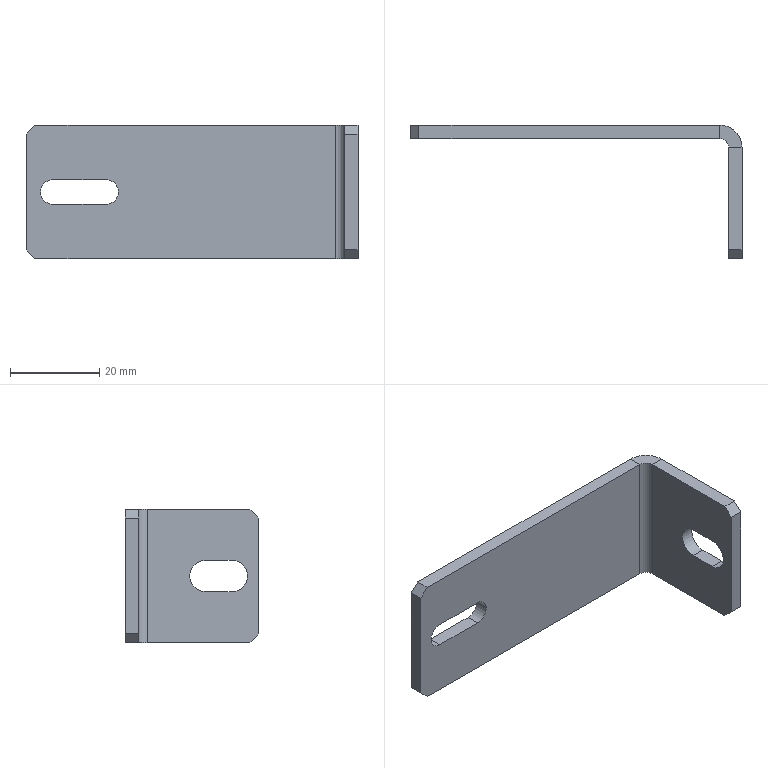Part | NX | features BREP 1 | 1 solid | 26 faces | box 74.5 x 30 x 30 mm | volume 8465 mm3 | plane 20 | cylinder 6 | commonest cylinder face diameters 5.5 x2 7 x2 4 x1 10 x1
STEP:
#1=CARTESIAN_POINT('',(74.5,-30.,-13.));
#2=VERTEX_POINT('',#1);
#3=CARTESIAN_POINT('',(74.5,-28.,-15.));
#4=VERTEX_POINT('',#3);
#5=CARTESIAN_POINT('',(74.5,-29.,-14.));
#6=DIRECTION('',(0.,0.7071,-0.7071));
#7=VECTOR('',#6,1000.);
#8=LINE('',#5,#7);
#9=EDGE_CURVE('',#2,#4,#8,.T.);
#10=ORIENTED_EDGE('',*,*,#9,.F.);
#11=CARTESIAN_POINT('',(71.5,-30.,-13.));
#12=VERTEX_POINT('',#11);
#13=CARTESIAN_POINT('',(74.5,-30.,-13.));
#14=DIRECTION('',(1.,0.,0.));
#15=VECTOR('',#14,1000.);
#16=LINE('',#13,#15);
#17=EDGE_CURVE('',#12,#2,#16,.T.);
#18=ORIENTED_EDGE('',*,*,#17,.F.);
#19=CARTESIAN_POINT('',(71.5,-28.,-15.));
#20=VERTEX_POINT('',#19);
#21=CARTESIAN_POINT('',(71.5,-28.,-15.));
#22=DIRECTION('',(0.,-0.7071,0.7071));
#23=VECTOR('',#22,1000.);
#24=LINE('',#21,#23);
#25=EDGE_CURVE('',#20,#12,#24,.T.);
#26=ORIENTED_EDGE('',*,*,#25,.F.);
#27=CARTESIAN_POINT('',(71.5,-28.,-15.));
#28=DIRECTION('',(-1.,0.,0.));
#29=VECTOR('',#28,1000.);
#30=LINE('',#27,#29);
#31=EDGE_CURVE('',#4,#20,#30,.T.);
#32=ORIENTED_EDGE('',*,*,#31,.F.);
#33=EDGE_LOOP('',(#10,#18,#26,#32));
#34=FACE_BOUND('',#33,.T.);
#35=CARTESIAN_POINT('',(69.5,-28.,-15.));
#36=DIRECTION('',(0.,-0.7071,-0.7071));
#37=DIRECTION('',(1.,0.,0.));
#38=AXIS2_PLACEMENT_3D('',#35,#36,#37);
#39=PLANE('',#38);
#40=ADVANCED_FACE('',(#34),#39,.T.);
#41=CARTESIAN_POINT('',(74.5,-28.,15.));
#42=VERTEX_POINT('',#41);
#43=CARTESIAN_POINT('',(74.5,-30.,13.));
#44=VERTEX_POINT('',#43);
#45=CARTESIAN_POINT('',(74.5,-14.,29.));
#46=DIRECTION('',(0.,-0.7071,-0.7071));
#47=VECTOR('',#46,1000.);
#48=LINE('',#45,#47);
#49=EDGE_CURVE('',#42,#44,#48,.T.);
#50=ORIENTED_EDGE('',*,*,#49,.F.);
#51=CARTESIAN_POINT('',(71.5,-28.,15.));
#52=VERTEX_POINT('',#51);
#53=CARTESIAN_POINT('',(69.5,-28.,15.));
#54=DIRECTION('',(1.,0.,0.));
#55=VECTOR('',#54,1000.);
#56=LINE('',#53,#55);
#57=EDGE_CURVE('',#52,#42,#56,.T.);
#58=ORIENTED_EDGE('',*,*,#57,.F.);
#59=CARTESIAN_POINT('',(71.5,-30.,13.));
#60=VERTEX_POINT('',#59);
#61=CARTESIAN_POINT('',(71.5,-30.,13.));
#62=DIRECTION('',(0.,0.7071,0.7071));
#63=VECTOR('',#62,1000.);
#64=LINE('',#61,#63);
#65=EDGE_CURVE('',#60,#52,#64,.T.);
#66=ORIENTED_EDGE('',*,*,#65,.F.);
#67=CARTESIAN_POINT('',(74.5,-30.,13.));
#68=DIRECTION('',(-1.,0.,0.));
#69=VECTOR('',#68,1000.);
#70=LINE('',#67,#69);
#71=EDGE_CURVE('',#44,#60,#70,.T.);
#72=ORIENTED_EDGE('',*,*,#71,.F.);
#73=EDGE_LOOP('',(#50,#58,#66,#72));
#74=FACE_BOUND('',#73,.T.);
#75=CARTESIAN_POINT('',(74.5,-30.,13.));
#76=DIRECTION('',(0.,0.7071,-0.7071));
#77=DIRECTION('',(-1.,0.,0.));
#78=AXIS2_PLACEMENT_3D('',#75,#76,#77);
#79=PLANE('',#78);
#80=ADVANCED_FACE('',(#74),#79,.F.);
#81=CARTESIAN_POINT('',(2.,-3.,15.));
#82=VERTEX_POINT('',#81);
#83=CARTESIAN_POINT('',(0.,-3.,13.));
#84=VERTEX_POINT('',#83);
#85=CARTESIAN_POINT('',(0.,-3.,13.));
#86=DIRECTION('',(-0.7071,0.,-0.7071));
#87=VECTOR('',#86,1000.);
#88=LINE('',#85,#87);
#89=EDGE_CURVE('',#82,#84,#88,.T.);
#90=ORIENTED_EDGE('',*,*,#89,.F.);
#91=CARTESIAN_POINT('',(2.,0.,15.));
#92=VERTEX_POINT('',#91);
#93=CARTESIAN_POINT('',(2.,-5.,15.));
#94=DIRECTION('',(0.,-1.,0.));
#95=VECTOR('',#94,1000.);
#96=LINE('',#93,#95);
#97=EDGE_CURVE('',#92,#82,#96,.T.);
#98=ORIENTED_EDGE('',*,*,#97,.F.);
#99=CARTESIAN_POINT('',(0.,0.,13.));
#100=VERTEX_POINT('',#99);
#101=CARTESIAN_POINT('',(1.,0.,14.));
#102=DIRECTION('',(0.7071,0.,0.7071));
#103=VECTOR('',#102,1000.);
#104=LINE('',#101,#103);
#105=EDGE_CURVE('',#100,#92,#104,.T.);
#106=ORIENTED_EDGE('',*,*,#105,.F.);
#107=CARTESIAN_POINT('',(0.,-3.,13.));
#108=DIRECTION('',(0.,1.,0.));
#109=VECTOR('',#108,1000.);
#110=LINE('',#107,#109);
#111=EDGE_CURVE('',#84,#100,#110,.T.);
#112=ORIENTED_EDGE('',*,*,#111,.F.);
#113=EDGE_LOOP('',(#90,#98,#106,#112));
#114=FACE_BOUND('',#113,.T.);
#115=CARTESIAN_POINT('',(0.,-3.,13.));
#116=DIRECTION('',(0.7071,0.,-0.7071));
#117=DIRECTION('',(0.,1.,0.));
#118=AXIS2_PLACEMENT_3D('',#115,#116,#117);
#119=PLANE('',#118);
#120=ADVANCED_FACE('',(#114),#119,.F.);
#121=CARTESIAN_POINT('',(0.,-3.,-13.));
#122=VERTEX_POINT('',#121);
#123=CARTESIAN_POINT('',(2.,-3.,-15.));
#124=VERTEX_POINT('',#123);
#125=CARTESIAN_POINT('',(2.,-3.,-15.));
#126=DIRECTION('',(0.7071,0.,-0.7071));
#127=VECTOR('',#126,1000.);
#128=LINE('',#125,#127);
#129=EDGE_CURVE('',#122,#124,#128,.T.);
#130=ORIENTED_EDGE('',*,*,#129,.F.);
#131=CARTESIAN_POINT('',(0.,0.,-13.));
#132=VERTEX_POINT('',#131);
#133=CARTESIAN_POINT('',(0.,-3.,-13.));
#134=DIRECTION('',(0.,-1.,0.));
#135=VECTOR('',#134,1000.);
#136=LINE('',#133,#135);
#137=EDGE_CURVE('',#132,#122,#136,.T.);
#138=ORIENTED_EDGE('',*,*,#137,.F.);
#139=CARTESIAN_POINT('',(2.,0.,-15.));
#140=VERTEX_POINT('',#139);
#141=CARTESIAN_POINT('',(-14.,0.,1.));
#142=DIRECTION('',(-0.7071,0.,0.7071));
#143=VECTOR('',#142,1000.);
#144=LINE('',#141,#143);
#145=EDGE_CURVE('',#140,#132,#144,.T.);
#146=ORIENTED_EDGE('',*,*,#145,.F.);
#147=CARTESIAN_POINT('',(2.,-5.,-15.));
#148=DIRECTION('',(0.,1.,0.));
#149=VECTOR('',#148,1000.);
#150=LINE('',#147,#149);
#151=EDGE_CURVE('',#124,#140,#150,.T.);
#152=ORIENTED_EDGE('',*,*,#151,.F.);
#153=EDGE_LOOP('',(#130,#138,#146,#152));
#154=FACE_BOUND('',#153,.T.);
#155=CARTESIAN_POINT('',(2.,-5.,-15.));
#156=DIRECTION('',(0.7071,0.,0.7071));
#157=DIRECTION('',(0.,1.,0.));
#158=AXIS2_PLACEMENT_3D('',#155,#156,#157);
#159=PLANE('',#158);
#160=ADVANCED_FACE('',(#154),#159,.F.);
#161=CARTESIAN_POINT('',(71.5,-24.,3.5));
#162=VERTEX_POINT('',#161);
#163=CARTESIAN_POINT('',(71.5,-18.,3.5));
#164=VERTEX_POINT('',#163);
#165=CARTESIAN_POINT('',(71.5,-24.,3.5));
#166=DIRECTION('',(0.,1.,0.));
#167=VECTOR('',#166,1000.);
#168=LINE('',#165,#167);
#169=EDGE_CURVE('',#162,#164,#168,.T.);
#170=ORIENTED_EDGE('',*,*,#169,.T.);
#171=CARTESIAN_POINT('',(74.5,-18.,3.5));
#172=VERTEX_POINT('',#171);
#173=CARTESIAN_POINT('',(74.5,-18.,3.5));
#174=DIRECTION('',(-1.,0.,0.));
#175=VECTOR('',#174,1000.);
#176=LINE('',#173,#175);
#177=EDGE_CURVE('',#172,#164,#176,.T.);
#178=ORIENTED_EDGE('',*,*,#177,.F.);
#179=CARTESIAN_POINT('',(74.5,-24.,3.5));
#180=VERTEX_POINT('',#179);
#181=CARTESIAN_POINT('',(74.5,-24.,3.5));
#182=DIRECTION('',(0.,1.,0.));
#183=VECTOR('',#182,1000.);
#184=LINE('',#181,#183);
#185=EDGE_CURVE('',#180,#172,#184,.T.);
#186=ORIENTED_EDGE('',*,*,#185,.F.);
#187=CARTESIAN_POINT('',(74.5,-24.,3.5));
#188=DIRECTION('',(-1.,0.,0.));
#189=VECTOR('',#188,1000.);
#190=LINE('',#187,#189);
#191=EDGE_CURVE('',#180,#162,#190,.T.);
#192=ORIENTED_EDGE('',*,*,#191,.T.);
#193=EDGE_LOOP('',(#170,#178,#186,#192));
#194=FACE_BOUND('',#193,.T.);
#195=CARTESIAN_POINT('',(74.5,-24.,3.5));
#196=DIRECTION('',(0.,0.,1.));
#197=DIRECTION('',(1.,0.,0.));
#198=AXIS2_PLACEMENT_3D('',#195,#196,#197);
#199=PLANE('',#198);
#200=ADVANCED_FACE('',(#194),#199,.F.);
#201=CARTESIAN_POINT('',(71.5,-18.,-3.5));
#202=VERTEX_POINT('',#201);
#203=CARTESIAN_POINT('',(71.5,-18.,0.));
#204=DIRECTION('',(-1.,0.,0.));
#205=DIRECTION('',(0.,0.,1.));
#206=AXIS2_PLACEMENT_3D('',#203,#204,#205);
#207=CIRCLE('',#206,3.5);
#208=EDGE_CURVE('',#164,#202,#207,.T.);
#209=ORIENTED_EDGE('',*,*,#208,.T.);
#210=CARTESIAN_POINT('',(74.5,-18.,-3.5));
#211=VERTEX_POINT('',#210);
#212=CARTESIAN_POINT('',(74.5,-18.,-3.5));
#213=DIRECTION('',(-1.,0.,0.));
#214=VECTOR('',#213,1000.);
#215=LINE('',#212,#214);
#216=EDGE_CURVE('',#211,#202,#215,.T.);
#217=ORIENTED_EDGE('',*,*,#216,.F.);
#218=CARTESIAN_POINT('',(74.5,-18.,0.));
#219=DIRECTION('',(-1.,0.,0.));
#220=DIRECTION('',(0.,0.,1.));
#221=AXIS2_PLACEMENT_3D('',#218,#219,#220);
#222=CIRCLE('',#221,3.5);
#223=EDGE_CURVE('',#172,#211,#222,.T.);
#224=ORIENTED_EDGE('',*,*,#223,.F.);
#225=ORIENTED_EDGE('',*,*,#177,.T.);
#226=EDGE_LOOP('',(#209,#217,#224,#225));
#227=FACE_BOUND('',#226,.T.);
#228=CARTESIAN_POINT('',(74.5,-18.,0.));
#229=DIRECTION('',(-1.,0.,0.));
#230=DIRECTION('',(0.,0.,1.));
#231=AXIS2_PLACEMENT_3D('',#228,#229,#230);
#232=CYLINDRICAL_SURFACE('',#231,3.5);
#233=ADVANCED_FACE('',(#227),#232,.F.);
#234=CARTESIAN_POINT('',(71.5,-24.,-3.5));
#235=VERTEX_POINT('',#234);
#236=CARTESIAN_POINT('',(71.5,-24.,-3.5));
#237=DIRECTION('',(0.,-1.,0.));
#238=VECTOR('',#237,1000.);
#239=LINE('',#236,#238);
#240=EDGE_CURVE('',#202,#235,#239,.T.);
#241=ORIENTED_EDGE('',*,*,#240,.T.);
#242=CARTESIAN_POINT('',(74.5,-24.,-3.5));
#243=VERTEX_POINT('',#242);
#244=CARTESIAN_POINT('',(74.5,-24.,-3.5));
#245=DIRECTION('',(-1.,0.,0.));
#246=VECTOR('',#245,1000.);
#247=LINE('',#244,#246);
#248=EDGE_CURVE('',#243,#235,#247,.T.);
#249=ORIENTED_EDGE('',*,*,#248,.F.);
#250=CARTESIAN_POINT('',(74.5,-24.,-3.5));
#251=DIRECTION('',(0.,-1.,0.));
#252=VECTOR('',#251,1000.);
#253=LINE('',#250,#252);
#254=EDGE_CURVE('',#211,#243,#253,.T.);
#255=ORIENTED_EDGE('',*,*,#254,.F.);
#256=ORIENTED_EDGE('',*,*,#216,.T.);
#257=EDGE_LOOP('',(#241,#249,#255,#256));
#258=FACE_BOUND('',#257,.T.);
#259=CARTESIAN_POINT('',(74.5,-24.,-3.5));
#260=DIRECTION('',(0.,0.,-1.));
#261=DIRECTION('',(-1.,0.,0.));
#262=AXIS2_PLACEMENT_3D('',#259,#260,#261);
#263=PLANE('',#262);
#264=ADVANCED_FACE('',(#258),#263,.F.);
#265=CARTESIAN_POINT('',(71.5,-24.,0.));
#266=DIRECTION('',(-1.,0.,0.));
#267=DIRECTION('',(0.,0.,1.));
#268=AXIS2_PLACEMENT_3D('',#265,#266,#267);
#269=CIRCLE('',#268,3.5);
#270=EDGE_CURVE('',#235,#162,#269,.T.);
#271=ORIENTED_EDGE('',*,*,#270,.T.);
#272=ORIENTED_EDGE('',*,*,#191,.F.);
#273=CARTESIAN_POINT('',(74.5,-24.,0.));
#274=DIRECTION('',(-1.,0.,0.));
#275=DIRECTION('',(0.,0.,1.));
#276=AXIS2_PLACEMENT_3D('',#273,#274,#275);
#277=CIRCLE('',#276,3.5);
#278=EDGE_CURVE('',#243,#180,#277,.T.);
#279=ORIENTED_EDGE('',*,*,#278,.F.);
#280=ORIENTED_EDGE('',*,*,#248,.T.);
#281=EDGE_LOOP('',(#271,#272,#279,#280));
#282=FACE_BOUND('',#281,.T.);
#283=CARTESIAN_POINT('',(74.5,-24.,0.));
#284=DIRECTION('',(-1.,0.,0.));
#285=DIRECTION('',(0.,0.,1.));
#286=AXIS2_PLACEMENT_3D('',#283,#284,#285);
#287=CYLINDRICAL_SURFACE('',#286,3.5);
#288=ADVANCED_FACE('',(#282),#287,.F.);
#289=CARTESIAN_POINT('',(6.,-3.,-2.75));
#290=VERTEX_POINT('',#289);
#291=CARTESIAN_POINT('',(18.,-3.,-2.75));
#292=VERTEX_POINT('',#291);
#293=CARTESIAN_POINT('',(6.,-3.,-2.75));
#294=DIRECTION('',(1.,0.,0.));
#295=VECTOR('',#294,1000.);
#296=LINE('',#293,#295);
#297=EDGE_CURVE('',#290,#292,#296,.T.);
#298=ORIENTED_EDGE('',*,*,#297,.T.);
#299=CARTESIAN_POINT('',(18.,0.,-2.75));
#300=VERTEX_POINT('',#299);
#301=CARTESIAN_POINT('',(18.,0.,-2.75));
#302=DIRECTION('',(0.,-1.,0.));
#303=VECTOR('',#302,1000.);
#304=LINE('',#301,#303);
#305=EDGE_CURVE('',#300,#292,#304,.T.);
#306=ORIENTED_EDGE('',*,*,#305,.F.);
#307=CARTESIAN_POINT('',(6.,0.,-2.75));
#308=VERTEX_POINT('',#307);
#309=CARTESIAN_POINT('',(6.,0.,-2.75));
#310=DIRECTION('',(1.,0.,0.));
#311=VECTOR('',#310,1000.);
#312=LINE('',#309,#311);
#313=EDGE_CURVE('',#308,#300,#312,.T.);
#314=ORIENTED_EDGE('',*,*,#313,.F.);
#315=CARTESIAN_POINT('',(6.,0.,-2.75));
#316=DIRECTION('',(0.,-1.,0.));
#317=VECTOR('',#316,1000.);
#318=LINE('',#315,#317);
#319=EDGE_CURVE('',#308,#290,#318,.T.);
#320=ORIENTED_EDGE('',*,*,#319,.T.);
#321=EDGE_LOOP('',(#298,#306,#314,#320));
#322=FACE_BOUND('',#321,.T.);
#323=CARTESIAN_POINT('',(6.,0.,-2.75));
#324=DIRECTION('',(0.,0.,-1.));
#325=DIRECTION('',(-1.,0.,0.));
#326=AXIS2_PLACEMENT_3D('',#323,#324,#325);
#327=PLANE('',#326);
#328=ADVANCED_FACE('',(#322),#327,.F.);
#329=CARTESIAN_POINT('',(18.,-3.,2.75));
#330=VERTEX_POINT('',#329);
#331=CARTESIAN_POINT('',(18.,-3.,0.));
#332=DIRECTION('',(0.,-1.,0.));
#333=DIRECTION('',(0.,0.,-1.));
#334=AXIS2_PLACEMENT_3D('',#331,#332,#333);
#335=CIRCLE('',#334,2.75);
#336=EDGE_CURVE('',#292,#330,#335,.T.);
#337=ORIENTED_EDGE('',*,*,#336,.T.);
#338=CARTESIAN_POINT('',(18.,0.,2.75));
#339=VERTEX_POINT('',#338);
#340=CARTESIAN_POINT('',(18.,0.,2.75));
#341=DIRECTION('',(0.,-1.,0.));
#342=VECTOR('',#341,1000.);
#343=LINE('',#340,#342);
#344=EDGE_CURVE('',#339,#330,#343,.T.);
#345=ORIENTED_EDGE('',*,*,#344,.F.);
#346=CARTESIAN_POINT('',(18.,0.,0.));
#347=DIRECTION('',(0.,-1.,0.));
#348=DIRECTION('',(0.,0.,-1.));
#349=AXIS2_PLACEMENT_3D('',#346,#347,#348);
#350=CIRCLE('',#349,2.75);
#351=EDGE_CURVE('',#300,#339,#350,.T.);
#352=ORIENTED_EDGE('',*,*,#351,.F.);
#353=ORIENTED_EDGE('',*,*,#305,.T.);
#354=EDGE_LOOP('',(#337,#345,#352,#353));
#355=FACE_BOUND('',#354,.T.);
#356=CARTESIAN_POINT('',(18.,0.,0.));
#357=DIRECTION('',(0.,-1.,0.));
#358=DIRECTION('',(0.,0.,-1.));
#359=AXIS2_PLACEMENT_3D('',#356,#357,#358);
#360=CYLINDRICAL_SURFACE('',#359,2.75);
#361=ADVANCED_FACE('',(#355),#360,.F.);
#362=CARTESIAN_POINT('',(6.,-3.,2.75));
#363=VERTEX_POINT('',#362);
#364=CARTESIAN_POINT('',(6.,-3.,2.75));
#365=DIRECTION('',(-1.,0.,0.));
#366=VECTOR('',#365,1000.);
#367=LINE('',#364,#366);
#368=EDGE_CURVE('',#330,#363,#367,.T.);
#369=ORIENTED_EDGE('',*,*,#368,.T.);
#370=CARTESIAN_POINT('',(6.,0.,2.75));
#371=VERTEX_POINT('',#370);
#372=CARTESIAN_POINT('',(6.,0.,2.75));
#373=DIRECTION('',(0.,-1.,0.));
#374=VECTOR('',#373,1000.);
#375=LINE('',#372,#374);
#376=EDGE_CURVE('',#371,#363,#375,.T.);
#377=ORIENTED_EDGE('',*,*,#376,.F.);
#378=CARTESIAN_POINT('',(6.,0.,2.75));
#379=DIRECTION('',(-1.,0.,0.));
#380=VECTOR('',#379,1000.);
#381=LINE('',#378,#380);
#382=EDGE_CURVE('',#339,#371,#381,.T.);
#383=ORIENTED_EDGE('',*,*,#382,.F.);
#384=ORIENTED_EDGE('',*,*,#344,.T.);
#385=EDGE_LOOP('',(#369,#377,#383,#384));
#386=FACE_BOUND('',#385,.T.);
#387=CARTESIAN_POINT('',(6.,0.,2.75));
#388=DIRECTION('',(0.,0.,1.));
#389=DIRECTION('',(1.,0.,0.));
#390=AXIS2_PLACEMENT_3D('',#387,#388,#389);
#391=PLANE('',#390);
#392=ADVANCED_FACE('',(#386),#391,.F.);
#393=CARTESIAN_POINT('',(6.,-3.,0.));
#394=DIRECTION('',(0.,-1.,0.));
#395=DIRECTION('',(0.,0.,-1.));
#396=AXIS2_PLACEMENT_3D('',#393,#394,#395);
#397=CIRCLE('',#396,2.75);
#398=EDGE_CURVE('',#363,#290,#397,.T.);
#399=ORIENTED_EDGE('',*,*,#398,.T.);
#400=ORIENTED_EDGE('',*,*,#319,.F.);
#401=CARTESIAN_POINT('',(6.,0.,0.));
#402=DIRECTION('',(0.,-1.,0.));
#403=DIRECTION('',(0.,0.,-1.));
#404=AXIS2_PLACEMENT_3D('',#401,#402,#403);
#405=CIRCLE('',#404,2.75);
#406=EDGE_CURVE('',#371,#308,#405,.T.);
#407=ORIENTED_EDGE('',*,*,#406,.F.);
#408=ORIENTED_EDGE('',*,*,#376,.T.);
#409=EDGE_LOOP('',(#399,#400,#407,#408));
#410=FACE_BOUND('',#409,.T.);
#411=CARTESIAN_POINT('',(6.,0.,0.));
#412=DIRECTION('',(0.,-1.,0.));
#413=DIRECTION('',(0.,0.,-1.));
#414=AXIS2_PLACEMENT_3D('',#411,#412,#413);
#415=CYLINDRICAL_SURFACE('',#414,2.75);
#416=ADVANCED_FACE('',(#410),#415,.F.);
#417=CARTESIAN_POINT('',(74.5,-5.,-15.));
#418=VERTEX_POINT('',#417);
#419=CARTESIAN_POINT('',(74.5,0.,-15.));
#420=DIRECTION('',(0.,-1.,0.));
#421=VECTOR('',#420,1000.);
#422=LINE('',#419,#421);
#423=EDGE_CURVE('',#418,#4,#422,.T.);
#424=ORIENTED_EDGE('',*,*,#423,.T.);
#425=ORIENTED_EDGE('',*,*,#31,.T.);
#426=CARTESIAN_POINT('',(71.5,-5.,-15.));
#427=VERTEX_POINT('',#426);
#428=CARTESIAN_POINT('',(71.5,0.,-15.));
#429=DIRECTION('',(0.,-1.,0.));
#430=VECTOR('',#429,1000.);
#431=LINE('',#428,#430);
#432=EDGE_CURVE('',#427,#20,#431,.T.);
#433=ORIENTED_EDGE('',*,*,#432,.F.);
#434=CARTESIAN_POINT('',(71.5,-5.,-15.));
#435=DIRECTION('',(1.,0.,0.));
#436=VECTOR('',#435,1000.);
#437=LINE('',#434,#436);
#438=EDGE_CURVE('',#427,#418,#437,.T.);
#439=ORIENTED_EDGE('',*,*,#438,.T.);
#440=EDGE_LOOP('',(#424,#425,#433,#439));
#441=FACE_BOUND('',#440,.T.);
#442=CARTESIAN_POINT('',(69.5,-5.,-15.));
#443=DIRECTION('',(0.,0.,1.));
#444=DIRECTION('',(1.,0.,0.));
#445=AXIS2_PLACEMENT_3D('',#442,#443,#444);
#446=PLANE('',#445);
#447=ADVANCED_FACE('',(#441),#446,.F.);
#448=CARTESIAN_POINT('',(69.5,0.,15.));
#449=VERTEX_POINT('',#448);
#450=CARTESIAN_POINT('',(0.,0.,15.));
#451=DIRECTION('',(1.,0.,0.));
#452=VECTOR('',#451,1000.);
#453=LINE('',#450,#452);
#454=EDGE_CURVE('',#92,#449,#453,.T.);
#455=ORIENTED_EDGE('',*,*,#454,.F.);
#456=ORIENTED_EDGE('',*,*,#97,.T.);
#457=CARTESIAN_POINT('',(69.5,-3.,15.));
#458=VERTEX_POINT('',#457);
#459=CARTESIAN_POINT('',(0.,-3.,15.));
#460=DIRECTION('',(1.,0.,0.));
#461=VECTOR('',#460,1000.);
#462=LINE('',#459,#461);
#463=EDGE_CURVE('',#82,#458,#462,.T.);
#464=ORIENTED_EDGE('',*,*,#463,.T.);
#465=CARTESIAN_POINT('',(69.5,-3.,15.));
#466=DIRECTION('',(0.,1.,0.));
#467=VECTOR('',#466,1000.);
#468=LINE('',#465,#467);
#469=EDGE_CURVE('',#458,#449,#468,.T.);
#470=ORIENTED_EDGE('',*,*,#469,.T.);
#471=EDGE_LOOP('',(#455,#456,#464,#470));
#472=FACE_BOUND('',#471,.T.);
#473=CARTESIAN_POINT('',(69.5,-5.,15.));
#474=DIRECTION('',(0.,0.,1.));
#475=DIRECTION('',(1.,0.,0.));
#476=AXIS2_PLACEMENT_3D('',#473,#474,#475);
#477=PLANE('',#476);
#478=ADVANCED_FACE('',(#472),#477,.T.);
#479=CARTESIAN_POINT('',(69.5,-3.,-15.));
#480=VERTEX_POINT('',#479);
#481=CARTESIAN_POINT('',(69.5,-5.,-15.));
#482=DIRECTION('',(0.,0.,-1.));
#483=DIRECTION('',(1.,0.,0.));
#484=AXIS2_PLACEMENT_3D('',#481,#482,#483);
#485=CIRCLE('',#484,2.);
#486=EDGE_CURVE('',#480,#427,#485,.T.);
#487=ORIENTED_EDGE('',*,*,#486,.T.);
#488=CARTESIAN_POINT('',(71.5,-5.,15.));
#489=VERTEX_POINT('',#488);
#490=CARTESIAN_POINT('',(71.5,-5.,15.));
#491=DIRECTION('',(0.,0.,-1.));
#492=VECTOR('',#491,1000.);
#493=LINE('',#490,#492);
#494=EDGE_CURVE('',#489,#427,#493,.T.);
#495=ORIENTED_EDGE('',*,*,#494,.F.);
#496=CARTESIAN_POINT('',(69.5,-5.,15.));
#497=DIRECTION('',(0.,0.,-1.));
#498=DIRECTION('',(1.,0.,0.));
#499=AXIS2_PLACEMENT_3D('',#496,#497,#498);
#500=CIRCLE('',#499,2.);
#501=EDGE_CURVE('',#458,#489,#500,.T.);
#502=ORIENTED_EDGE('',*,*,#501,.F.);
#503=CARTESIAN_POINT('',(69.5,-3.,15.));
#504=DIRECTION('',(0.,0.,-1.));
#505=VECTOR('',#504,1000.);
#506=LINE('',#503,#505);
#507=EDGE_CURVE('',#458,#480,#506,.T.);
#508=ORIENTED_EDGE('',*,*,#507,.T.);
#509=EDGE_LOOP('',(#487,#495,#502,#508));
#510=FACE_BOUND('',#509,.T.);
#511=CARTESIAN_POINT('',(69.5,-5.,15.));
#512=DIRECTION('',(0.,0.,-1.));
#513=DIRECTION('',(-1.,0.,0.));
#514=AXIS2_PLACEMENT_3D('',#511,#512,#513);
#515=CYLINDRICAL_SURFACE('',#514,2.);
#516=ADVANCED_FACE('',(#510),#515,.F.);
#517=CARTESIAN_POINT('',(0.,-3.,15.));
#518=DIRECTION('',(0.,0.,-1.));
#519=VECTOR('',#518,1000.);
#520=LINE('',#517,#519);
#521=EDGE_CURVE('',#84,#122,#520,.T.);
#522=ORIENTED_EDGE('',*,*,#521,.T.);
#523=ORIENTED_EDGE('',*,*,#129,.T.);
#524=CARTESIAN_POINT('',(0.,-3.,-15.));
#525=DIRECTION('',(1.,0.,0.));
#526=VECTOR('',#525,1000.);
#527=LINE('',#524,#526);
#528=EDGE_CURVE('',#124,#480,#527,.T.);
#529=ORIENTED_EDGE('',*,*,#528,.T.);
#530=ORIENTED_EDGE('',*,*,#507,.F.);
#531=ORIENTED_EDGE('',*,*,#463,.F.);
#532=ORIENTED_EDGE('',*,*,#89,.T.);
#533=EDGE_LOOP('',(#522,#523,#529,#530,#531,#532));
#534=FACE_BOUND('',#533,.T.);
#535=ORIENTED_EDGE('',*,*,#297,.F.);
#536=ORIENTED_EDGE('',*,*,#398,.F.);
#537=ORIENTED_EDGE('',*,*,#368,.F.);
#538=ORIENTED_EDGE('',*,*,#336,.F.);
#539=EDGE_LOOP('',(#535,#536,#537,#538));
#540=FACE_BOUND('',#539,.T.);
#541=CARTESIAN_POINT('',(0.,-3.,15.));
#542=DIRECTION('',(0.,1.,0.));
#543=DIRECTION('',(0.,0.,1.));
#544=AXIS2_PLACEMENT_3D('',#541,#542,#543);
#545=PLANE('',#544);
#546=ADVANCED_FACE('',(#534,#540),#545,.F.);
#547=CARTESIAN_POINT('',(0.,0.,15.));
#548=DIRECTION('',(0.,0.,-1.));
#549=VECTOR('',#548,1000.);
#550=LINE('',#547,#549);
#551=EDGE_CURVE('',#100,#132,#550,.T.);
#552=ORIENTED_EDGE('',*,*,#551,.T.);
#553=ORIENTED_EDGE('',*,*,#137,.T.);
#554=ORIENTED_EDGE('',*,*,#521,.F.);
#555=ORIENTED_EDGE('',*,*,#111,.T.);
#556=EDGE_LOOP('',(#552,#553,#554,#555));
#557=FACE_BOUND('',#556,.T.);
#558=CARTESIAN_POINT('',(0.,-3.,15.));
#559=DIRECTION('',(-1.,0.,0.));
#560=DIRECTION('',(0.,0.,1.));
#561=AXIS2_PLACEMENT_3D('',#558,#559,#560);
#562=PLANE('',#561);
#563=ADVANCED_FACE('',(#557),#562,.T.);
#564=CARTESIAN_POINT('',(69.5,0.,-15.));
#565=VERTEX_POINT('',#564);
#566=CARTESIAN_POINT('',(0.,0.,-15.));
#567=DIRECTION('',(1.,0.,0.));
#568=VECTOR('',#567,1000.);
#569=LINE('',#566,#568);
#570=EDGE_CURVE('',#140,#565,#569,.T.);
#571=ORIENTED_EDGE('',*,*,#570,.F.);
#572=ORIENTED_EDGE('',*,*,#145,.T.);
#573=ORIENTED_EDGE('',*,*,#551,.F.);
#574=ORIENTED_EDGE('',*,*,#105,.T.);
#575=ORIENTED_EDGE('',*,*,#454,.T.);
#576=CARTESIAN_POINT('',(69.5,0.,15.));
#577=DIRECTION('',(0.,0.,-1.));
#578=VECTOR('',#577,1000.);
#579=LINE('',#576,#578);
#580=EDGE_CURVE('',#449,#565,#579,.T.);
#581=ORIENTED_EDGE('',*,*,#580,.T.);
#582=EDGE_LOOP('',(#571,#572,#573,#574,#575,#581));
#583=FACE_BOUND('',#582,.T.);
#584=ORIENTED_EDGE('',*,*,#406,.T.);
#585=ORIENTED_EDGE('',*,*,#313,.T.);
#586=ORIENTED_EDGE('',*,*,#351,.T.);
#587=ORIENTED_EDGE('',*,*,#382,.T.);
#588=EDGE_LOOP('',(#584,#585,#586,#587));
#589=FACE_BOUND('',#588,.T.);
#590=CARTESIAN_POINT('',(0.,0.,15.));
#591=DIRECTION('',(0.,1.,0.));
#592=DIRECTION('',(0.,0.,1.));
#593=AXIS2_PLACEMENT_3D('',#590,#591,#592);
#594=PLANE('',#593);
#595=ADVANCED_FACE('',(#583,#589),#594,.T.);
#596=CARTESIAN_POINT('',(69.5,-5.,-15.));
#597=DIRECTION('',(0.,0.,-1.));
#598=DIRECTION('',(1.,0.,0.));
#599=AXIS2_PLACEMENT_3D('',#596,#597,#598);
#600=CIRCLE('',#599,5.);
#601=EDGE_CURVE('',#565,#418,#600,.T.);
#602=ORIENTED_EDGE('',*,*,#601,.F.);
#603=ORIENTED_EDGE('',*,*,#580,.F.);
#604=CARTESIAN_POINT('',(74.5,-5.,15.));
#605=VERTEX_POINT('',#604);
#606=CARTESIAN_POINT('',(69.5,-5.,15.));
#607=DIRECTION('',(0.,0.,-1.));
#608=DIRECTION('',(1.,0.,0.));
#609=AXIS2_PLACEMENT_3D('',#606,#607,#608);
#610=CIRCLE('',#609,5.);
#611=EDGE_CURVE('',#449,#605,#610,.T.);
#612=ORIENTED_EDGE('',*,*,#611,.T.);
#613=CARTESIAN_POINT('',(74.5,-5.,15.));
#614=DIRECTION('',(0.,0.,-1.));
#615=VECTOR('',#614,1000.);
#616=LINE('',#613,#615);
#617=EDGE_CURVE('',#605,#418,#616,.T.);
#618=ORIENTED_EDGE('',*,*,#617,.T.);
#619=EDGE_LOOP('',(#602,#603,#612,#618));
#620=FACE_BOUND('',#619,.T.);
#621=CARTESIAN_POINT('',(69.5,-5.,15.));
#622=DIRECTION('',(0.,0.,-1.));
#623=DIRECTION('',(-1.,0.,0.));
#624=AXIS2_PLACEMENT_3D('',#621,#622,#623);
#625=CYLINDRICAL_SURFACE('',#624,5.);
#626=ADVANCED_FACE('',(#620),#625,.T.);
#627=CARTESIAN_POINT('',(74.5,0.,15.));
#628=DIRECTION('',(0.,-1.,0.));
#629=VECTOR('',#628,1000.);
#630=LINE('',#627,#629);
#631=EDGE_CURVE('',#605,#42,#630,.T.);
#632=ORIENTED_EDGE('',*,*,#631,.T.);
#633=ORIENTED_EDGE('',*,*,#49,.T.);
#634=CARTESIAN_POINT('',(74.5,-30.,15.));
#635=DIRECTION('',(0.,0.,-1.));
#636=VECTOR('',#635,1000.);
#637=LINE('',#634,#636);
#638=EDGE_CURVE('',#44,#2,#637,.T.);
#639=ORIENTED_EDGE('',*,*,#638,.T.);
#640=ORIENTED_EDGE('',*,*,#9,.T.);
#641=ORIENTED_EDGE('',*,*,#423,.F.);
#642=ORIENTED_EDGE('',*,*,#617,.F.);
#643=EDGE_LOOP('',(#632,#633,#639,#640,#641,#642));
#644=FACE_BOUND('',#643,.T.);
#645=ORIENTED_EDGE('',*,*,#278,.T.);
#646=ORIENTED_EDGE('',*,*,#185,.T.);
#647=ORIENTED_EDGE('',*,*,#223,.T.);
#648=ORIENTED_EDGE('',*,*,#254,.T.);
#649=EDGE_LOOP('',(#645,#646,#647,#648));
#650=FACE_BOUND('',#649,.T.);
#651=CARTESIAN_POINT('',(74.5,0.,15.));
#652=DIRECTION('',(1.,0.,0.));
#653=DIRECTION('',(0.,0.,-1.));
#654=AXIS2_PLACEMENT_3D('',#651,#652,#653);
#655=PLANE('',#654);
#656=ADVANCED_FACE('',(#644,#650),#655,.T.);
#657=ORIENTED_EDGE('',*,*,#638,.F.);
#658=ORIENTED_EDGE('',*,*,#71,.T.);
#659=CARTESIAN_POINT('',(71.5,-30.,15.));
#660=DIRECTION('',(0.,0.,-1.));
#661=VECTOR('',#660,1000.);
#662=LINE('',#659,#661);
#663=EDGE_CURVE('',#60,#12,#662,.T.);
#664=ORIENTED_EDGE('',*,*,#663,.T.);
#665=ORIENTED_EDGE('',*,*,#17,.T.);
#666=EDGE_LOOP('',(#657,#658,#664,#665));
#667=FACE_BOUND('',#666,.T.);
#668=CARTESIAN_POINT('',(74.5,-30.,15.));
#669=DIRECTION('',(0.,-1.,0.));
#670=DIRECTION('',(0.,0.,-1.));
#671=AXIS2_PLACEMENT_3D('',#668,#669,#670);
#672=PLANE('',#671);
#673=ADVANCED_FACE('',(#667),#672,.T.);
#674=ORIENTED_EDGE('',*,*,#663,.F.);
#675=ORIENTED_EDGE('',*,*,#65,.T.);
#676=CARTESIAN_POINT('',(71.5,0.,15.));
#677=DIRECTION('',(0.,-1.,0.));
#678=VECTOR('',#677,1000.);
#679=LINE('',#676,#678);
#680=EDGE_CURVE('',#489,#52,#679,.T.);
#681=ORIENTED_EDGE('',*,*,#680,.F.);
#682=ORIENTED_EDGE('',*,*,#494,.T.);
#683=ORIENTED_EDGE('',*,*,#432,.T.);
#684=ORIENTED_EDGE('',*,*,#25,.T.);
#685=EDGE_LOOP('',(#674,#675,#681,#682,#683,#684));
#686=FACE_BOUND('',#685,.T.);
#687=ORIENTED_EDGE('',*,*,#169,.F.);
#688=ORIENTED_EDGE('',*,*,#270,.F.);
#689=ORIENTED_EDGE('',*,*,#240,.F.);
#690=ORIENTED_EDGE('',*,*,#208,.F.);
#691=EDGE_LOOP('',(#687,#688,#689,#690));
#692=FACE_BOUND('',#691,.T.);
#693=CARTESIAN_POINT('',(71.5,0.,15.));
#694=DIRECTION('',(1.,0.,0.));
#695=DIRECTION('',(0.,0.,-1.));
#696=AXIS2_PLACEMENT_3D('',#693,#694,#695);
#697=PLANE('',#696);
#698=ADVANCED_FACE('',(#686,#692),#697,.F.);
#699=ORIENTED_EDGE('',*,*,#528,.F.);
#700=ORIENTED_EDGE('',*,*,#151,.T.);
#701=ORIENTED_EDGE('',*,*,#570,.T.);
#702=CARTESIAN_POINT('',(69.5,0.,-15.));
#703=DIRECTION('',(0.,-1.,0.));
#704=VECTOR('',#703,1000.);
#705=LINE('',#702,#704);
#706=EDGE_CURVE('',#565,#480,#705,.T.);
#707=ORIENTED_EDGE('',*,*,#706,.T.);
#708=EDGE_LOOP('',(#699,#700,#701,#707));
#709=FACE_BOUND('',#708,.T.);
#710=CARTESIAN_POINT('',(71.5,-5.,-15.));
#711=DIRECTION('',(0.,0.,-1.));
#712=DIRECTION('',(-1.,0.,0.));
#713=AXIS2_PLACEMENT_3D('',#710,#711,#712);
#714=PLANE('',#713);
#715=ADVANCED_FACE('',(#709),#714,.T.);
#716=ORIENTED_EDGE('',*,*,#706,.F.);
#717=ORIENTED_EDGE('',*,*,#601,.T.);
#718=ORIENTED_EDGE('',*,*,#438,.F.);
#719=ORIENTED_EDGE('',*,*,#486,.F.);
#720=EDGE_LOOP('',(#716,#717,#718,#719));
#721=FACE_BOUND('',#720,.T.);
#722=CARTESIAN_POINT('',(69.5,0.,-15.));
#723=DIRECTION('',(0.,0.,-1.));
#724=DIRECTION('',(-1.,0.,0.));
#725=AXIS2_PLACEMENT_3D('',#722,#723,#724);
#726=PLANE('',#725);
#727=ADVANCED_FACE('',(#721),#726,.T.);
#728=ORIENTED_EDGE('',*,*,#680,.T.);
#729=ORIENTED_EDGE('',*,*,#57,.T.);
#730=ORIENTED_EDGE('',*,*,#631,.F.);
#731=CARTESIAN_POINT('',(74.5,-5.,15.));
#732=DIRECTION('',(-1.,0.,0.));
#733=VECTOR('',#732,1000.);
#734=LINE('',#731,#733);
#735=EDGE_CURVE('',#605,#489,#734,.T.);
#736=ORIENTED_EDGE('',*,*,#735,.T.);
#737=EDGE_LOOP('',(#728,#729,#730,#736));
#738=FACE_BOUND('',#737,.T.);
#739=CARTESIAN_POINT('',(69.5,-3.,15.));
#740=DIRECTION('',(0.,0.,1.));
#741=DIRECTION('',(1.,0.,0.));
#742=AXIS2_PLACEMENT_3D('',#739,#740,#741);
#743=PLANE('',#742);
#744=ADVANCED_FACE('',(#738),#743,.T.);
#745=ORIENTED_EDGE('',*,*,#735,.F.);
#746=ORIENTED_EDGE('',*,*,#611,.F.);
#747=ORIENTED_EDGE('',*,*,#469,.F.);
#748=ORIENTED_EDGE('',*,*,#501,.T.);
#749=EDGE_LOOP('',(#745,#746,#747,#748));
#750=FACE_BOUND('',#749,.T.);
#751=CARTESIAN_POINT('',(74.5,-5.,15.));
#752=DIRECTION('',(0.,0.,1.));
#753=DIRECTION('',(1.,0.,0.));
#754=AXIS2_PLACEMENT_3D('',#751,#752,#753);
#755=PLANE('',#754);
#756=ADVANCED_FACE('',(#750),#755,.T.);
#757=CLOSED_SHELL('',(#40,#80,#120,#160,#200,#233,#264,#288,#328,#361,#392,#416,#447,#478,#516,#546,#563,#595,#626,#656,#673,#698,#715,#727,#744,#756));
#758=MANIFOLD_SOLID_BREP('',#757);
#759=(LENGTH_UNIT()NAMED_UNIT(*)SI_UNIT(.MILLI.,.METRE.));
#760=UNCERTAINTY_MEASURE_WITH_UNIT(LENGTH_MEASURE(0.00001),#759,'','');
#761=(NAMED_UNIT(*)PLANE_ANGLE_UNIT()SI_UNIT($,.RADIAN.));
#762=(NAMED_UNIT(*)SI_UNIT($,.STERADIAN.)SOLID_ANGLE_UNIT());
#763=(GEOMETRIC_REPRESENTATION_CONTEXT(3)GLOBAL_UNCERTAINTY_ASSIGNED_CONTEXT((#760))GLOBAL_UNIT_ASSIGNED_CONTEXT((#759,#761,#762))REPRESENTATION_CONTEXT('',''));
#764=ADVANCED_BREP_SHAPE_REPRESENTATION('',(#758),#763);